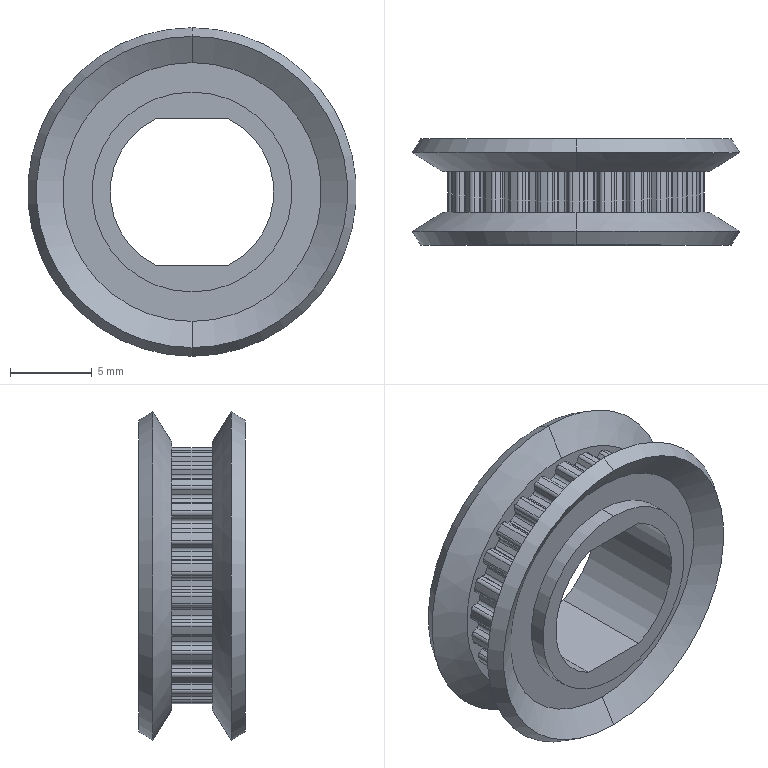Part | NX | features BREP 1 | 1 solid | 246 faces | box 20.061 x 6.5 x 20.061 mm | volume 821.799 mm3 | cylinder 151 | plane 83 | cone 12 | commonest cylinder face diameters 0.46 x120 15.66 x25 12.2 x4 10 x2